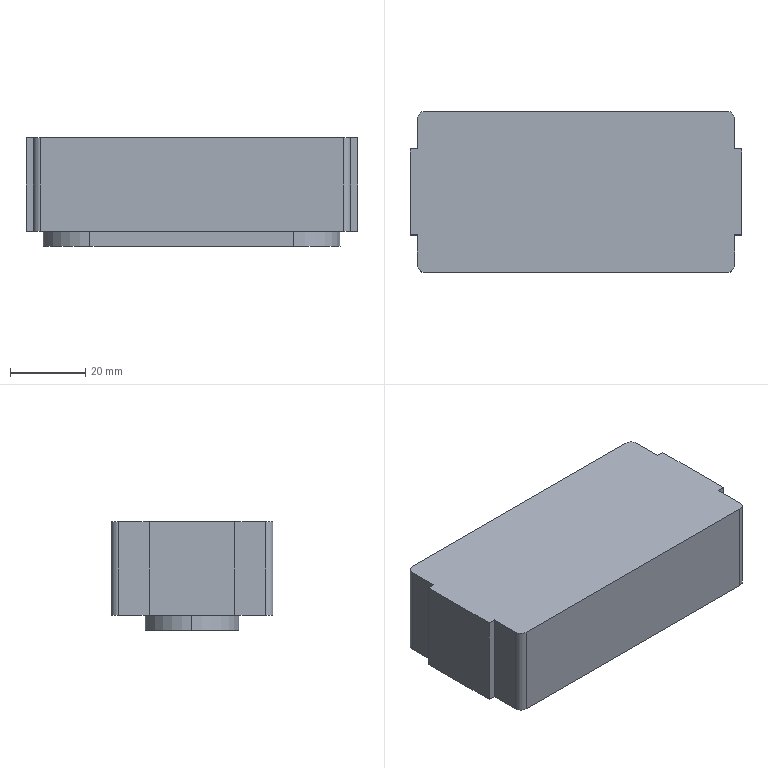Part | SolidWorks | features Extrusion 1, Fillet 1, ICE 1 | 1 solid | 24 faces | box 88.335 x 43.022 x 29 mm | volume 100368 mm3 | plane 17 | cylinder 7 | commonest cylinder face diameters 4 x4 24.966 x3
STEP:
#1=CARTESIAN_POINT('',(-39.672,0.,4.));
#2=VERTEX_POINT('',#1);
#3=CARTESIAN_POINT('',(-27.189,-12.483,4.));
#4=VERTEX_POINT('',#3);
#5=CARTESIAN_POINT('',(-27.189,0.,4.));
#6=DIRECTION('',(0.,0.,1.));
#7=DIRECTION('',(1.,0.,0.));
#8=AXIS2_PLACEMENT_3D('',#5,#6,#7);
#9=CIRCLE('',#8,12.483);
#10=EDGE_CURVE('',#2,#4,#9,.T.);
#11=ORIENTED_EDGE('',*,*,#10,.F.);
#12=CARTESIAN_POINT('',(-39.672,0.,0.));
#13=VERTEX_POINT('',#12);
#14=CARTESIAN_POINT('',(-39.672,0.,4.));
#15=DIRECTION('',(0.,0.,-1.));
#16=VECTOR('',#15,1000.);
#17=LINE('',#14,#16);
#18=EDGE_CURVE('',#2,#13,#17,.T.);
#19=ORIENTED_EDGE('',*,*,#18,.T.);
#20=CARTESIAN_POINT('',(-27.189,-12.483,0.));
#21=VERTEX_POINT('',#20);
#22=CARTESIAN_POINT('',(-27.189,0.,0.));
#23=DIRECTION('',(0.,0.,1.));
#24=DIRECTION('',(1.,0.,0.));
#25=AXIS2_PLACEMENT_3D('',#22,#23,#24);
#26=CIRCLE('',#25,12.483);
#27=EDGE_CURVE('',#13,#21,#26,.T.);
#28=ORIENTED_EDGE('',*,*,#27,.T.);
#29=CARTESIAN_POINT('',(-27.189,-12.483,4.));
#30=DIRECTION('',(0.,0.,-1.));
#31=VECTOR('',#30,1000.);
#32=LINE('',#29,#31);
#33=EDGE_CURVE('',#4,#21,#32,.T.);
#34=ORIENTED_EDGE('',*,*,#33,.F.);
#35=EDGE_LOOP('',(#11,#19,#28,#34));
#36=FACE_OUTER_BOUND('',#35,.T.);
#37=CARTESIAN_POINT('',(-27.189,0.,4.));
#38=DIRECTION('',(0.,0.,-1.));
#39=DIRECTION('',(-1.,0.,0.));
#40=AXIS2_PLACEMENT_3D('',#37,#38,#39);
#41=CYLINDRICAL_SURFACE('',#40,12.483);
#42=ADVANCED_FACE('',(#36),#41,.T.);
#43=CARTESIAN_POINT('',(27.066,-12.483,0.));
#44=VERTEX_POINT('',#43);
#45=CARTESIAN_POINT('',(27.066,12.483,0.));
#46=VERTEX_POINT('',#45);
#47=CARTESIAN_POINT('',(27.066,0.,0.));
#48=DIRECTION('',(0.,0.,1.));
#49=DIRECTION('',(1.,0.,0.));
#50=AXIS2_PLACEMENT_3D('',#47,#48,#49);
#51=CIRCLE('',#50,12.483);
#52=EDGE_CURVE('',#44,#46,#51,.T.);
#53=ORIENTED_EDGE('',*,*,#52,.T.);
#54=CARTESIAN_POINT('',(27.066,12.483,4.));
#55=VERTEX_POINT('',#54);
#56=CARTESIAN_POINT('',(27.066,12.483,4.));
#57=DIRECTION('',(0.,0.,-1.));
#58=VECTOR('',#57,1000.);
#59=LINE('',#56,#58);
#60=EDGE_CURVE('',#55,#46,#59,.T.);
#61=ORIENTED_EDGE('',*,*,#60,.F.);
#62=CARTESIAN_POINT('',(27.066,-12.483,4.));
#63=VERTEX_POINT('',#62);
#64=CARTESIAN_POINT('',(27.066,0.,4.));
#65=DIRECTION('',(0.,0.,1.));
#66=DIRECTION('',(1.,0.,0.));
#67=AXIS2_PLACEMENT_3D('',#64,#65,#66);
#68=CIRCLE('',#67,12.483);
#69=EDGE_CURVE('',#63,#55,#68,.T.);
#70=ORIENTED_EDGE('',*,*,#69,.F.);
#71=CARTESIAN_POINT('',(27.066,-12.483,4.));
#72=DIRECTION('',(0.,0.,-1.));
#73=VECTOR('',#72,1000.);
#74=LINE('',#71,#73);
#75=EDGE_CURVE('',#63,#44,#74,.T.);
#76=ORIENTED_EDGE('',*,*,#75,.T.);
#77=EDGE_LOOP('',(#53,#61,#70,#76));
#78=FACE_OUTER_BOUND('',#77,.T.);
#79=CARTESIAN_POINT('',(27.066,0.,4.));
#80=DIRECTION('',(0.,0.,-1.));
#81=DIRECTION('',(-1.,0.,0.));
#82=AXIS2_PLACEMENT_3D('',#79,#80,#81);
#83=CYLINDRICAL_SURFACE('',#82,12.483);
#84=ADVANCED_FACE('',(#78),#83,.T.);
#85=CARTESIAN_POINT('',(-27.189,12.483,0.));
#86=VERTEX_POINT('',#85);
#87=CARTESIAN_POINT('',(27.066,12.483,0.));
#88=DIRECTION('',(-1.,0.,0.));
#89=VECTOR('',#88,1000.);
#90=LINE('',#87,#89);
#91=EDGE_CURVE('',#46,#86,#90,.T.);
#92=ORIENTED_EDGE('',*,*,#91,.T.);
#93=CARTESIAN_POINT('',(-27.189,12.483,4.));
#94=VERTEX_POINT('',#93);
#95=CARTESIAN_POINT('',(-27.189,12.483,4.));
#96=DIRECTION('',(0.,0.,-1.));
#97=VECTOR('',#96,1000.);
#98=LINE('',#95,#97);
#99=EDGE_CURVE('',#94,#86,#98,.T.);
#100=ORIENTED_EDGE('',*,*,#99,.F.);
#101=CARTESIAN_POINT('',(27.066,12.483,4.));
#102=DIRECTION('',(-1.,0.,0.));
#103=VECTOR('',#102,1000.);
#104=LINE('',#101,#103);
#105=EDGE_CURVE('',#55,#94,#104,.T.);
#106=ORIENTED_EDGE('',*,*,#105,.F.);
#107=ORIENTED_EDGE('',*,*,#60,.T.);
#108=EDGE_LOOP('',(#92,#100,#106,#107));
#109=FACE_OUTER_BOUND('',#108,.T.);
#110=CARTESIAN_POINT('',(27.066,12.483,4.));
#111=DIRECTION('',(0.,-1.,0.));
#112=DIRECTION('',(1.,0.,0.));
#113=AXIS2_PLACEMENT_3D('',#110,#111,#112);
#114=PLANE('',#113);
#115=ADVANCED_FACE('',(#109),#114,.F.);
#116=ORIENTED_EDGE('',*,*,#18,.F.);
#117=CARTESIAN_POINT('',(-27.189,0.,4.));
#118=DIRECTION('',(0.,0.,1.));
#119=DIRECTION('',(1.,0.,0.));
#120=AXIS2_PLACEMENT_3D('',#117,#118,#119);
#121=CIRCLE('',#120,12.483);
#122=EDGE_CURVE('',#94,#2,#121,.T.);
#123=ORIENTED_EDGE('',*,*,#122,.F.);
#124=ORIENTED_EDGE('',*,*,#99,.T.);
#125=CARTESIAN_POINT('',(-27.189,0.,0.));
#126=DIRECTION('',(0.,0.,1.));
#127=DIRECTION('',(1.,0.,0.));
#128=AXIS2_PLACEMENT_3D('',#125,#126,#127);
#129=CIRCLE('',#128,12.483);
#130=EDGE_CURVE('',#86,#13,#129,.T.);
#131=ORIENTED_EDGE('',*,*,#130,.T.);
#132=EDGE_LOOP('',(#116,#123,#124,#131));
#133=FACE_OUTER_BOUND('',#132,.T.);
#134=CARTESIAN_POINT('',(-27.189,0.,4.));
#135=DIRECTION('',(0.,0.,-1.));
#136=DIRECTION('',(-1.,0.,0.));
#137=AXIS2_PLACEMENT_3D('',#134,#135,#136);
#138=CYLINDRICAL_SURFACE('',#137,12.483);
#139=ADVANCED_FACE('',(#133),#138,.T.);
#140=CARTESIAN_POINT('',(27.066,-12.483,0.));
#141=DIRECTION('',(1.,0.,0.));
#142=VECTOR('',#141,1000.);
#143=LINE('',#140,#142);
#144=EDGE_CURVE('',#21,#44,#143,.T.);
#145=ORIENTED_EDGE('',*,*,#144,.T.);
#146=ORIENTED_EDGE('',*,*,#75,.F.);
#147=CARTESIAN_POINT('',(27.066,-12.483,4.));
#148=DIRECTION('',(1.,0.,0.));
#149=VECTOR('',#148,1000.);
#150=LINE('',#147,#149);
#151=EDGE_CURVE('',#4,#63,#150,.T.);
#152=ORIENTED_EDGE('',*,*,#151,.F.);
#153=ORIENTED_EDGE('',*,*,#33,.T.);
#154=EDGE_LOOP('',(#145,#146,#152,#153));
#155=FACE_OUTER_BOUND('',#154,.T.);
#156=CARTESIAN_POINT('',(27.066,-12.483,4.));
#157=DIRECTION('',(0.,1.,0.));
#158=DIRECTION('',(-1.,0.,0.));
#159=AXIS2_PLACEMENT_3D('',#156,#157,#158);
#160=PLANE('',#159);
#161=ADVANCED_FACE('',(#155),#160,.F.);
#162=ORIENTED_EDGE('',*,*,#52,.F.);
#163=ORIENTED_EDGE('',*,*,#144,.F.);
#164=ORIENTED_EDGE('',*,*,#27,.F.);
#165=ORIENTED_EDGE('',*,*,#130,.F.);
#166=ORIENTED_EDGE('',*,*,#91,.F.);
#167=EDGE_LOOP('',(#162,#163,#164,#165,#166));
#168=FACE_OUTER_BOUND('',#167,.T.);
#169=CARTESIAN_POINT('',(27.066,0.,0.));
#170=DIRECTION('',(0.,0.,1.));
#171=DIRECTION('',(1.,0.,0.));
#172=AXIS2_PLACEMENT_3D('',#169,#170,#171);
#173=PLANE('',#172);
#174=ADVANCED_FACE('',(#168),#173,.F.);
#175=CARTESIAN_POINT('',(-42.249,19.511,4.));
#176=VERTEX_POINT('',#175);
#177=CARTESIAN_POINT('',(-42.249,11.445,4.));
#178=VERTEX_POINT('',#177);
#179=CARTESIAN_POINT('',(-42.249,11.445,4.));
#180=DIRECTION('',(0.,-1.,0.));
#181=VECTOR('',#180,1000.);
#182=LINE('',#179,#181);
#183=EDGE_CURVE('',#176,#178,#182,.T.);
#184=ORIENTED_EDGE('',*,*,#183,.F.);
#185=CARTESIAN_POINT('',(-40.249,21.511,4.));
#186=VERTEX_POINT('',#185);
#187=CARTESIAN_POINT('',(-40.249,19.511,4.));
#188=DIRECTION('',(0.,0.,-1.));
#189=DIRECTION('',(1.,0.,0.));
#190=AXIS2_PLACEMENT_3D('',#187,#188,#189);
#191=CIRCLE('',#190,2.);
#192=EDGE_CURVE('',#176,#186,#191,.T.);
#193=ORIENTED_EDGE('',*,*,#192,.T.);
#194=CARTESIAN_POINT('',(40.249,21.511,4.));
#195=VERTEX_POINT('',#194);
#196=CARTESIAN_POINT('',(42.249,21.511,4.));
#197=DIRECTION('',(-1.,0.,0.));
#198=VECTOR('',#197,1000.);
#199=LINE('',#196,#198);
#200=EDGE_CURVE('',#195,#186,#199,.T.);
#201=ORIENTED_EDGE('',*,*,#200,.F.);
#202=CARTESIAN_POINT('',(42.249,19.511,4.));
#203=VERTEX_POINT('',#202);
#204=CARTESIAN_POINT('',(40.249,19.511,4.));
#205=DIRECTION('',(0.,0.,-1.));
#206=DIRECTION('',(1.,0.,0.));
#207=AXIS2_PLACEMENT_3D('',#204,#205,#206);
#208=CIRCLE('',#207,2.);
#209=EDGE_CURVE('',#195,#203,#208,.T.);
#210=ORIENTED_EDGE('',*,*,#209,.T.);
#211=CARTESIAN_POINT('',(42.249,11.445,4.));
#212=VERTEX_POINT('',#211);
#213=CARTESIAN_POINT('',(42.249,11.445,4.));
#214=DIRECTION('',(0.,1.,0.));
#215=VECTOR('',#214,1000.);
#216=LINE('',#213,#215);
#217=EDGE_CURVE('',#212,#203,#216,.T.);
#218=ORIENTED_EDGE('',*,*,#217,.F.);
#219=CARTESIAN_POINT('',(44.167,11.445,4.));
#220=VERTEX_POINT('',#219);
#221=CARTESIAN_POINT('',(44.167,11.445,4.));
#222=DIRECTION('',(-1.,0.,0.));
#223=VECTOR('',#222,1000.);
#224=LINE('',#221,#223);
#225=EDGE_CURVE('',#220,#212,#224,.T.);
#226=ORIENTED_EDGE('',*,*,#225,.F.);
#227=CARTESIAN_POINT('',(44.167,-11.445,4.));
#228=VERTEX_POINT('',#227);
#229=CARTESIAN_POINT('',(44.167,-11.445,4.));
#230=DIRECTION('',(0.,1.,0.));
#231=VECTOR('',#230,1000.);
#232=LINE('',#229,#231);
#233=EDGE_CURVE('',#228,#220,#232,.T.);
#234=ORIENTED_EDGE('',*,*,#233,.F.);
#235=CARTESIAN_POINT('',(42.249,-11.445,4.));
#236=VERTEX_POINT('',#235);
#237=CARTESIAN_POINT('',(44.167,-11.445,4.));
#238=DIRECTION('',(1.,0.,0.));
#239=VECTOR('',#238,1000.);
#240=LINE('',#237,#239);
#241=EDGE_CURVE('',#236,#228,#240,.T.);
#242=ORIENTED_EDGE('',*,*,#241,.F.);
#243=CARTESIAN_POINT('',(42.249,-19.511,4.));
#244=VERTEX_POINT('',#243);
#245=CARTESIAN_POINT('',(42.249,-21.511,4.));
#246=DIRECTION('',(0.,1.,0.));
#247=VECTOR('',#246,1000.);
#248=LINE('',#245,#247);
#249=EDGE_CURVE('',#244,#236,#248,.T.);
#250=ORIENTED_EDGE('',*,*,#249,.F.);
#251=CARTESIAN_POINT('',(40.249,-21.511,4.));
#252=VERTEX_POINT('',#251);
#253=CARTESIAN_POINT('',(40.249,-19.511,4.));
#254=DIRECTION('',(0.,0.,-1.));
#255=DIRECTION('',(1.,0.,0.));
#256=AXIS2_PLACEMENT_3D('',#253,#254,#255);
#257=CIRCLE('',#256,2.);
#258=EDGE_CURVE('',#244,#252,#257,.T.);
#259=ORIENTED_EDGE('',*,*,#258,.T.);
#260=CARTESIAN_POINT('',(-40.249,-21.511,4.));
#261=VERTEX_POINT('',#260);
#262=CARTESIAN_POINT('',(42.249,-21.511,4.));
#263=DIRECTION('',(1.,0.,0.));
#264=VECTOR('',#263,1000.);
#265=LINE('',#262,#264);
#266=EDGE_CURVE('',#261,#252,#265,.T.);
#267=ORIENTED_EDGE('',*,*,#266,.F.);
#268=CARTESIAN_POINT('',(-42.249,-19.511,4.));
#269=VERTEX_POINT('',#268);
#270=CARTESIAN_POINT('',(-40.249,-19.511,4.));
#271=DIRECTION('',(0.,0.,-1.));
#272=DIRECTION('',(1.,0.,0.));
#273=AXIS2_PLACEMENT_3D('',#270,#271,#272);
#274=CIRCLE('',#273,2.);
#275=EDGE_CURVE('',#261,#269,#274,.T.);
#276=ORIENTED_EDGE('',*,*,#275,.T.);
#277=CARTESIAN_POINT('',(-42.249,-11.445,4.));
#278=VERTEX_POINT('',#277);
#279=CARTESIAN_POINT('',(-42.249,-21.511,4.));
#280=DIRECTION('',(0.,-1.,0.));
#281=VECTOR('',#280,1000.);
#282=LINE('',#279,#281);
#283=EDGE_CURVE('',#278,#269,#282,.T.);
#284=ORIENTED_EDGE('',*,*,#283,.F.);
#285=CARTESIAN_POINT('',(-44.167,-11.445,4.));
#286=VERTEX_POINT('',#285);
#287=CARTESIAN_POINT('',(-44.167,-11.445,4.));
#288=DIRECTION('',(1.,0.,0.));
#289=VECTOR('',#288,1000.);
#290=LINE('',#287,#289);
#291=EDGE_CURVE('',#286,#278,#290,.T.);
#292=ORIENTED_EDGE('',*,*,#291,.F.);
#293=CARTESIAN_POINT('',(-44.167,11.445,4.));
#294=VERTEX_POINT('',#293);
#295=CARTESIAN_POINT('',(-44.167,-11.445,4.));
#296=DIRECTION('',(0.,-1.,0.));
#297=VECTOR('',#296,1000.);
#298=LINE('',#295,#297);
#299=EDGE_CURVE('',#294,#286,#298,.T.);
#300=ORIENTED_EDGE('',*,*,#299,.F.);
#301=CARTESIAN_POINT('',(-44.167,11.445,4.));
#302=DIRECTION('',(-1.,0.,0.));
#303=VECTOR('',#302,1000.);
#304=LINE('',#301,#303);
#305=EDGE_CURVE('',#178,#294,#304,.T.);
#306=ORIENTED_EDGE('',*,*,#305,.F.);
#307=EDGE_LOOP('',(#184,#193,#201,#210,#218,#226,#234,#242,#250,#259,#267,#276,#284,#292,#300,#306));
#308=FACE_OUTER_BOUND('',#307,.T.);
#309=ORIENTED_EDGE('',*,*,#151,.T.);
#310=ORIENTED_EDGE('',*,*,#69,.T.);
#311=ORIENTED_EDGE('',*,*,#105,.T.);
#312=ORIENTED_EDGE('',*,*,#122,.T.);
#313=ORIENTED_EDGE('',*,*,#10,.T.);
#314=EDGE_LOOP('',(#309,#310,#311,#312,#313));
#315=FACE_BOUND('',#314,.T.);
#316=CARTESIAN_POINT('',(0.,0.,4.));
#317=DIRECTION('',(0.,0.,1.));
#318=DIRECTION('',(1.,0.,0.));
#319=AXIS2_PLACEMENT_3D('',#316,#317,#318);
#320=PLANE('',#319);
#321=ADVANCED_FACE('',(#308,#315),#320,.F.);
#322=CARTESIAN_POINT('',(-42.249,19.511,29.));
#323=VERTEX_POINT('',#322);
#324=CARTESIAN_POINT('',(-42.249,11.445,29.));
#325=VERTEX_POINT('',#324);
#326=CARTESIAN_POINT('',(-42.249,11.445,29.));
#327=DIRECTION('',(0.,-1.,0.));
#328=VECTOR('',#327,1000.);
#329=LINE('',#326,#328);
#330=EDGE_CURVE('',#323,#325,#329,.T.);
#331=ORIENTED_EDGE('',*,*,#330,.F.);
#332=CARTESIAN_POINT('',(-42.249,19.511,29.));
#333=DIRECTION('',(0.,0.,-1.));
#334=VECTOR('',#333,1000.);
#335=LINE('',#332,#334);
#336=EDGE_CURVE('',#323,#176,#335,.T.);
#337=ORIENTED_EDGE('',*,*,#336,.T.);
#338=ORIENTED_EDGE('',*,*,#183,.T.);
#339=CARTESIAN_POINT('',(-42.249,11.445,29.));
#340=DIRECTION('',(0.,0.,-1.));
#341=VECTOR('',#340,1000.);
#342=LINE('',#339,#341);
#343=EDGE_CURVE('',#325,#178,#342,.T.);
#344=ORIENTED_EDGE('',*,*,#343,.F.);
#345=EDGE_LOOP('',(#331,#337,#338,#344));
#346=FACE_OUTER_BOUND('',#345,.T.);
#347=CARTESIAN_POINT('',(-42.249,11.445,29.));
#348=DIRECTION('',(1.,0.,0.));
#349=DIRECTION('',(0.,0.,-1.));
#350=AXIS2_PLACEMENT_3D('',#347,#348,#349);
#351=PLANE('',#350);
#352=ADVANCED_FACE('',(#346),#351,.F.);
#353=ORIENTED_EDGE('',*,*,#305,.T.);
#354=CARTESIAN_POINT('',(-44.167,11.445,29.));
#355=VERTEX_POINT('',#354);
#356=CARTESIAN_POINT('',(-44.167,11.445,29.));
#357=DIRECTION('',(0.,0.,-1.));
#358=VECTOR('',#357,1000.);
#359=LINE('',#356,#358);
#360=EDGE_CURVE('',#355,#294,#359,.T.);
#361=ORIENTED_EDGE('',*,*,#360,.F.);
#362=CARTESIAN_POINT('',(-44.167,11.445,29.));
#363=DIRECTION('',(-1.,0.,0.));
#364=VECTOR('',#363,1000.);
#365=LINE('',#362,#364);
#366=EDGE_CURVE('',#325,#355,#365,.T.);
#367=ORIENTED_EDGE('',*,*,#366,.F.);
#368=ORIENTED_EDGE('',*,*,#343,.T.);
#369=EDGE_LOOP('',(#353,#361,#367,#368));
#370=FACE_OUTER_BOUND('',#369,.T.);
#371=CARTESIAN_POINT('',(-44.167,11.445,29.));
#372=DIRECTION('',(0.,-1.,0.));
#373=DIRECTION('',(1.,0.,0.));
#374=AXIS2_PLACEMENT_3D('',#371,#372,#373);
#375=PLANE('',#374);
#376=ADVANCED_FACE('',(#370),#375,.F.);
#377=ORIENTED_EDGE('',*,*,#299,.T.);
#378=CARTESIAN_POINT('',(-44.167,-11.445,29.));
#379=VERTEX_POINT('',#378);
#380=CARTESIAN_POINT('',(-44.167,-11.445,29.));
#381=DIRECTION('',(0.,0.,-1.));
#382=VECTOR('',#381,1000.);
#383=LINE('',#380,#382);
#384=EDGE_CURVE('',#379,#286,#383,.T.);
#385=ORIENTED_EDGE('',*,*,#384,.F.);
#386=CARTESIAN_POINT('',(-44.167,-11.445,29.));
#387=DIRECTION('',(0.,-1.,0.));
#388=VECTOR('',#387,1000.);
#389=LINE('',#386,#388);
#390=EDGE_CURVE('',#355,#379,#389,.T.);
#391=ORIENTED_EDGE('',*,*,#390,.F.);
#392=ORIENTED_EDGE('',*,*,#360,.T.);
#393=EDGE_LOOP('',(#377,#385,#391,#392));
#394=FACE_OUTER_BOUND('',#393,.T.);
#395=CARTESIAN_POINT('',(-44.167,-11.445,29.));
#396=DIRECTION('',(1.,0.,0.));
#397=DIRECTION('',(0.,0.,-1.));
#398=AXIS2_PLACEMENT_3D('',#395,#396,#397);
#399=PLANE('',#398);
#400=ADVANCED_FACE('',(#394),#399,.F.);
#401=ORIENTED_EDGE('',*,*,#291,.T.);
#402=CARTESIAN_POINT('',(-42.249,-11.445,29.));
#403=VERTEX_POINT('',#402);
#404=CARTESIAN_POINT('',(-42.249,-11.445,29.));
#405=DIRECTION('',(0.,0.,-1.));
#406=VECTOR('',#405,1000.);
#407=LINE('',#404,#406);
#408=EDGE_CURVE('',#403,#278,#407,.T.);
#409=ORIENTED_EDGE('',*,*,#408,.F.);
#410=CARTESIAN_POINT('',(-44.167,-11.445,29.));
#411=DIRECTION('',(1.,0.,0.));
#412=VECTOR('',#411,1000.);
#413=LINE('',#410,#412);
#414=EDGE_CURVE('',#379,#403,#413,.T.);
#415=ORIENTED_EDGE('',*,*,#414,.F.);
#416=ORIENTED_EDGE('',*,*,#384,.T.);
#417=EDGE_LOOP('',(#401,#409,#415,#416));
#418=FACE_OUTER_BOUND('',#417,.T.);
#419=CARTESIAN_POINT('',(-44.167,-11.445,29.));
#420=DIRECTION('',(0.,1.,0.));
#421=DIRECTION('',(0.,0.,1.));
#422=AXIS2_PLACEMENT_3D('',#419,#420,#421);
#423=PLANE('',#422);
#424=ADVANCED_FACE('',(#418),#423,.F.);
#425=ORIENTED_EDGE('',*,*,#283,.T.);
#426=CARTESIAN_POINT('',(-42.249,-19.511,29.));
#427=VERTEX_POINT('',#426);
#428=CARTESIAN_POINT('',(-42.249,-19.511,29.));
#429=DIRECTION('',(0.,0.,1.));
#430=VECTOR('',#429,1000.);
#431=LINE('',#428,#430);
#432=EDGE_CURVE('',#269,#427,#431,.T.);
#433=ORIENTED_EDGE('',*,*,#432,.T.);
#434=CARTESIAN_POINT('',(-42.249,-21.511,29.));
#435=DIRECTION('',(0.,-1.,0.));
#436=VECTOR('',#435,1000.);
#437=LINE('',#434,#436);
#438=EDGE_CURVE('',#403,#427,#437,.T.);
#439=ORIENTED_EDGE('',*,*,#438,.F.);
#440=ORIENTED_EDGE('',*,*,#408,.T.);
#441=EDGE_LOOP('',(#425,#433,#439,#440));
#442=FACE_OUTER_BOUND('',#441,.T.);
#443=CARTESIAN_POINT('',(-42.249,-21.511,29.));
#444=DIRECTION('',(1.,0.,0.));
#445=DIRECTION('',(0.,0.,-1.));
#446=AXIS2_PLACEMENT_3D('',#443,#444,#445);
#447=PLANE('',#446);
#448=ADVANCED_FACE('',(#442),#447,.F.);
#449=CARTESIAN_POINT('',(-40.249,-21.511,29.));
#450=VERTEX_POINT('',#449);
#451=CARTESIAN_POINT('',(40.249,-21.511,29.));
#452=VERTEX_POINT('',#451);
#453=CARTESIAN_POINT('',(42.249,-21.511,29.));
#454=DIRECTION('',(1.,0.,0.));
#455=VECTOR('',#454,1000.);
#456=LINE('',#453,#455);
#457=EDGE_CURVE('',#450,#452,#456,.T.);
#458=ORIENTED_EDGE('',*,*,#457,.F.);
#459=CARTESIAN_POINT('',(-40.249,-21.511,29.));
#460=DIRECTION('',(0.,0.,-1.));
#461=VECTOR('',#460,1000.);
#462=LINE('',#459,#461);
#463=EDGE_CURVE('',#450,#261,#462,.T.);
#464=ORIENTED_EDGE('',*,*,#463,.T.);
#465=ORIENTED_EDGE('',*,*,#266,.T.);
#466=CARTESIAN_POINT('',(40.249,-21.511,29.));
#467=DIRECTION('',(0.,0.,1.));
#468=VECTOR('',#467,1000.);
#469=LINE('',#466,#468);
#470=EDGE_CURVE('',#252,#452,#469,.T.);
#471=ORIENTED_EDGE('',*,*,#470,.T.);
#472=EDGE_LOOP('',(#458,#464,#465,#471));
#473=FACE_OUTER_BOUND('',#472,.T.);
#474=CARTESIAN_POINT('',(42.249,-21.511,29.));
#475=DIRECTION('',(0.,1.,0.));
#476=DIRECTION('',(0.,0.,1.));
#477=AXIS2_PLACEMENT_3D('',#474,#475,#476);
#478=PLANE('',#477);
#479=ADVANCED_FACE('',(#473),#478,.F.);
#480=CARTESIAN_POINT('',(42.249,-19.511,29.));
#481=VERTEX_POINT('',#480);
#482=CARTESIAN_POINT('',(42.249,-11.445,29.));
#483=VERTEX_POINT('',#482);
#484=CARTESIAN_POINT('',(42.249,-21.511,29.));
#485=DIRECTION('',(0.,1.,0.));
#486=VECTOR('',#485,1000.);
#487=LINE('',#484,#486);
#488=EDGE_CURVE('',#481,#483,#487,.T.);
#489=ORIENTED_EDGE('',*,*,#488,.F.);
#490=CARTESIAN_POINT('',(42.249,-19.511,29.));
#491=DIRECTION('',(0.,0.,-1.));
#492=VECTOR('',#491,1000.);
#493=LINE('',#490,#492);
#494=EDGE_CURVE('',#481,#244,#493,.T.);
#495=ORIENTED_EDGE('',*,*,#494,.T.);
#496=ORIENTED_EDGE('',*,*,#249,.T.);
#497=CARTESIAN_POINT('',(42.249,-11.445,29.));
#498=DIRECTION('',(0.,0.,-1.));
#499=VECTOR('',#498,1000.);
#500=LINE('',#497,#499);
#501=EDGE_CURVE('',#483,#236,#500,.T.);
#502=ORIENTED_EDGE('',*,*,#501,.F.);
#503=EDGE_LOOP('',(#489,#495,#496,#502));
#504=FACE_OUTER_BOUND('',#503,.T.);
#505=CARTESIAN_POINT('',(42.249,-21.511,29.));
#506=DIRECTION('',(-1.,0.,0.));
#507=DIRECTION('',(0.,0.,1.));
#508=AXIS2_PLACEMENT_3D('',#505,#506,#507);
#509=PLANE('',#508);
#510=ADVANCED_FACE('',(#504),#509,.F.);
#511=ORIENTED_EDGE('',*,*,#241,.T.);
#512=CARTESIAN_POINT('',(44.167,-11.445,29.));
#513=VERTEX_POINT('',#512);
#514=CARTESIAN_POINT('',(44.167,-11.445,29.));
#515=DIRECTION('',(0.,0.,-1.));
#516=VECTOR('',#515,1000.);
#517=LINE('',#514,#516);
#518=EDGE_CURVE('',#513,#228,#517,.T.);
#519=ORIENTED_EDGE('',*,*,#518,.F.);
#520=CARTESIAN_POINT('',(44.167,-11.445,29.));
#521=DIRECTION('',(1.,0.,0.));
#522=VECTOR('',#521,1000.);
#523=LINE('',#520,#522);
#524=EDGE_CURVE('',#483,#513,#523,.T.);
#525=ORIENTED_EDGE('',*,*,#524,.F.);
#526=ORIENTED_EDGE('',*,*,#501,.T.);
#527=EDGE_LOOP('',(#511,#519,#525,#526));
#528=FACE_OUTER_BOUND('',#527,.T.);
#529=CARTESIAN_POINT('',(44.167,-11.445,29.));
#530=DIRECTION('',(0.,1.,0.));
#531=DIRECTION('',(0.,0.,1.));
#532=AXIS2_PLACEMENT_3D('',#529,#530,#531);
#533=PLANE('',#532);
#534=ADVANCED_FACE('',(#528),#533,.F.);
#535=ORIENTED_EDGE('',*,*,#233,.T.);
#536=CARTESIAN_POINT('',(44.167,11.445,29.));
#537=VERTEX_POINT('',#536);
#538=CARTESIAN_POINT('',(44.167,11.445,29.));
#539=DIRECTION('',(0.,0.,-1.));
#540=VECTOR('',#539,1000.);
#541=LINE('',#538,#540);
#542=EDGE_CURVE('',#537,#220,#541,.T.);
#543=ORIENTED_EDGE('',*,*,#542,.F.);
#544=CARTESIAN_POINT('',(44.167,-11.445,29.));
#545=DIRECTION('',(0.,1.,0.));
#546=VECTOR('',#545,1000.);
#547=LINE('',#544,#546);
#548=EDGE_CURVE('',#513,#537,#547,.T.);
#549=ORIENTED_EDGE('',*,*,#548,.F.);
#550=ORIENTED_EDGE('',*,*,#518,.T.);
#551=EDGE_LOOP('',(#535,#543,#549,#550));
#552=FACE_OUTER_BOUND('',#551,.T.);
#553=CARTESIAN_POINT('',(44.167,-11.445,29.));
#554=DIRECTION('',(-1.,0.,0.));
#555=DIRECTION('',(0.,0.,1.));
#556=AXIS2_PLACEMENT_3D('',#553,#554,#555);
#557=PLANE('',#556);
#558=ADVANCED_FACE('',(#552),#557,.F.);
#559=ORIENTED_EDGE('',*,*,#225,.T.);
#560=CARTESIAN_POINT('',(42.249,11.445,29.));
#561=VERTEX_POINT('',#560);
#562=CARTESIAN_POINT('',(42.249,11.445,29.));
#563=DIRECTION('',(0.,0.,-1.));
#564=VECTOR('',#563,1000.);
#565=LINE('',#562,#564);
#566=EDGE_CURVE('',#561,#212,#565,.T.);
#567=ORIENTED_EDGE('',*,*,#566,.F.);
#568=CARTESIAN_POINT('',(44.167,11.445,29.));
#569=DIRECTION('',(-1.,0.,0.));
#570=VECTOR('',#569,1000.);
#571=LINE('',#568,#570);
#572=EDGE_CURVE('',#537,#561,#571,.T.);
#573=ORIENTED_EDGE('',*,*,#572,.F.);
#574=ORIENTED_EDGE('',*,*,#542,.T.);
#575=EDGE_LOOP('',(#559,#567,#573,#574));
#576=FACE_OUTER_BOUND('',#575,.T.);
#577=CARTESIAN_POINT('',(44.167,11.445,29.));
#578=DIRECTION('',(0.,-1.,0.));
#579=DIRECTION('',(1.,0.,0.));
#580=AXIS2_PLACEMENT_3D('',#577,#578,#579);
#581=PLANE('',#580);
#582=ADVANCED_FACE('',(#576),#581,.F.);
#583=ORIENTED_EDGE('',*,*,#217,.T.);
#584=CARTESIAN_POINT('',(42.249,19.511,29.));
#585=VERTEX_POINT('',#584);
#586=CARTESIAN_POINT('',(42.249,19.511,29.));
#587=DIRECTION('',(0.,0.,1.));
#588=VECTOR('',#587,1000.);
#589=LINE('',#586,#588);
#590=EDGE_CURVE('',#203,#585,#589,.T.);
#591=ORIENTED_EDGE('',*,*,#590,.T.);
#592=CARTESIAN_POINT('',(42.249,11.445,29.));
#593=DIRECTION('',(0.,1.,0.));
#594=VECTOR('',#593,1000.);
#595=LINE('',#592,#594);
#596=EDGE_CURVE('',#561,#585,#595,.T.);
#597=ORIENTED_EDGE('',*,*,#596,.F.);
#598=ORIENTED_EDGE('',*,*,#566,.T.);
#599=EDGE_LOOP('',(#583,#591,#597,#598));
#600=FACE_OUTER_BOUND('',#599,.T.);
#601=CARTESIAN_POINT('',(42.249,11.445,29.));
#602=DIRECTION('',(-1.,0.,0.));
#603=DIRECTION('',(0.,0.,1.));
#604=AXIS2_PLACEMENT_3D('',#601,#602,#603);
#605=PLANE('',#604);
#606=ADVANCED_FACE('',(#600),#605,.F.);
#607=ORIENTED_EDGE('',*,*,#200,.T.);
#608=CARTESIAN_POINT('',(-40.249,21.511,29.));
#609=VERTEX_POINT('',#608);
#610=CARTESIAN_POINT('',(-40.249,21.511,29.));
#611=DIRECTION('',(0.,0.,1.));
#612=VECTOR('',#611,1000.);
#613=LINE('',#610,#612);
#614=EDGE_CURVE('',#186,#609,#613,.T.);
#615=ORIENTED_EDGE('',*,*,#614,.T.);
#616=CARTESIAN_POINT('',(40.249,21.511,29.));
#617=VERTEX_POINT('',#616);
#618=CARTESIAN_POINT('',(42.249,21.511,29.));
#619=DIRECTION('',(-1.,0.,0.));
#620=VECTOR('',#619,1000.);
#621=LINE('',#618,#620);
#622=EDGE_CURVE('',#617,#609,#621,.T.);
#623=ORIENTED_EDGE('',*,*,#622,.F.);
#624=CARTESIAN_POINT('',(40.249,21.511,29.));
#625=DIRECTION('',(0.,0.,-1.));
#626=VECTOR('',#625,1000.);
#627=LINE('',#624,#626);
#628=EDGE_CURVE('',#617,#195,#627,.T.);
#629=ORIENTED_EDGE('',*,*,#628,.T.);
#630=EDGE_LOOP('',(#607,#615,#623,#629));
#631=FACE_OUTER_BOUND('',#630,.T.);
#632=CARTESIAN_POINT('',(42.249,21.511,29.));
#633=DIRECTION('',(0.,-1.,0.));
#634=DIRECTION('',(0.,0.,-1.));
#635=AXIS2_PLACEMENT_3D('',#632,#633,#634);
#636=PLANE('',#635);
#637=ADVANCED_FACE('',(#631),#636,.F.);
#638=ORIENTED_EDGE('',*,*,#622,.T.);
#639=CARTESIAN_POINT('',(-40.249,19.511,29.));
#640=DIRECTION('',(0.,0.,1.));
#641=DIRECTION('',(1.,0.,0.));
#642=AXIS2_PLACEMENT_3D('',#639,#640,#641);
#643=CIRCLE('',#642,2.);
#644=EDGE_CURVE('',#609,#323,#643,.T.);
#645=ORIENTED_EDGE('',*,*,#644,.T.);
#646=ORIENTED_EDGE('',*,*,#330,.T.);
#647=ORIENTED_EDGE('',*,*,#366,.T.);
#648=ORIENTED_EDGE('',*,*,#390,.T.);
#649=ORIENTED_EDGE('',*,*,#414,.T.);
#650=ORIENTED_EDGE('',*,*,#438,.T.);
#651=CARTESIAN_POINT('',(-40.249,-19.511,29.));
#652=DIRECTION('',(0.,0.,1.));
#653=DIRECTION('',(1.,0.,0.));
#654=AXIS2_PLACEMENT_3D('',#651,#652,#653);
#655=CIRCLE('',#654,2.);
#656=EDGE_CURVE('',#427,#450,#655,.T.);
#657=ORIENTED_EDGE('',*,*,#656,.T.);
#658=ORIENTED_EDGE('',*,*,#457,.T.);
#659=CARTESIAN_POINT('',(40.249,-19.511,29.));
#660=DIRECTION('',(0.,0.,1.));
#661=DIRECTION('',(1.,0.,0.));
#662=AXIS2_PLACEMENT_3D('',#659,#660,#661);
#663=CIRCLE('',#662,2.);
#664=EDGE_CURVE('',#452,#481,#663,.T.);
#665=ORIENTED_EDGE('',*,*,#664,.T.);
#666=ORIENTED_EDGE('',*,*,#488,.T.);
#667=ORIENTED_EDGE('',*,*,#524,.T.);
#668=ORIENTED_EDGE('',*,*,#548,.T.);
#669=ORIENTED_EDGE('',*,*,#572,.T.);
#670=ORIENTED_EDGE('',*,*,#596,.T.);
#671=CARTESIAN_POINT('',(40.249,19.511,29.));
#672=DIRECTION('',(0.,0.,1.));
#673=DIRECTION('',(1.,0.,0.));
#674=AXIS2_PLACEMENT_3D('',#671,#672,#673);
#675=CIRCLE('',#674,2.);
#676=EDGE_CURVE('',#585,#617,#675,.T.);
#677=ORIENTED_EDGE('',*,*,#676,.T.);
#678=EDGE_LOOP('',(#638,#645,#646,#647,#648,#649,#650,#657,#658,#665,#666,#667,#668,#669,#670,#677));
#679=FACE_OUTER_BOUND('',#678,.T.);
#680=CARTESIAN_POINT('',(0.,0.,29.));
#681=DIRECTION('',(0.,0.,1.));
#682=DIRECTION('',(1.,0.,0.));
#683=AXIS2_PLACEMENT_3D('',#680,#681,#682);
#684=PLANE('',#683);
#685=ADVANCED_FACE('',(#679),#684,.T.);
#686=ORIENTED_EDGE('',*,*,#644,.F.);
#687=ORIENTED_EDGE('',*,*,#614,.F.);
#688=ORIENTED_EDGE('',*,*,#192,.F.);
#689=ORIENTED_EDGE('',*,*,#336,.F.);
#690=EDGE_LOOP('',(#686,#687,#688,#689));
#691=FACE_OUTER_BOUND('',#690,.T.);
#692=CARTESIAN_POINT('',(-40.249,19.511,29.));
#693=DIRECTION('',(0.,0.,-1.));
#694=DIRECTION('',(-1.,0.,0.));
#695=AXIS2_PLACEMENT_3D('',#692,#693,#694);
#696=CYLINDRICAL_SURFACE('',#695,2.);
#697=ADVANCED_FACE('',(#691),#696,.T.);
#698=ORIENTED_EDGE('',*,*,#656,.F.);
#699=ORIENTED_EDGE('',*,*,#432,.F.);
#700=ORIENTED_EDGE('',*,*,#275,.F.);
#701=ORIENTED_EDGE('',*,*,#463,.F.);
#702=EDGE_LOOP('',(#698,#699,#700,#701));
#703=FACE_OUTER_BOUND('',#702,.T.);
#704=CARTESIAN_POINT('',(-40.249,-19.511,29.));
#705=DIRECTION('',(0.,0.,-1.));
#706=DIRECTION('',(-1.,0.,0.));
#707=AXIS2_PLACEMENT_3D('',#704,#705,#706);
#708=CYLINDRICAL_SURFACE('',#707,2.);
#709=ADVANCED_FACE('',(#703),#708,.T.);
#710=ORIENTED_EDGE('',*,*,#676,.F.);
#711=ORIENTED_EDGE('',*,*,#590,.F.);
#712=ORIENTED_EDGE('',*,*,#209,.F.);
#713=ORIENTED_EDGE('',*,*,#628,.F.);
#714=EDGE_LOOP('',(#710,#711,#712,#713));
#715=FACE_OUTER_BOUND('',#714,.T.);
#716=CARTESIAN_POINT('',(40.249,19.511,29.));
#717=DIRECTION('',(0.,0.,-1.));
#718=DIRECTION('',(-1.,0.,0.));
#719=AXIS2_PLACEMENT_3D('',#716,#717,#718);
#720=CYLINDRICAL_SURFACE('',#719,2.);
#721=ADVANCED_FACE('',(#715),#720,.T.);
#722=ORIENTED_EDGE('',*,*,#664,.F.);
#723=ORIENTED_EDGE('',*,*,#470,.F.);
#724=ORIENTED_EDGE('',*,*,#258,.F.);
#725=ORIENTED_EDGE('',*,*,#494,.F.);
#726=EDGE_LOOP('',(#722,#723,#724,#725));
#727=FACE_OUTER_BOUND('',#726,.T.);
#728=CARTESIAN_POINT('',(40.249,-19.511,29.));
#729=DIRECTION('',(0.,0.,-1.));
#730=DIRECTION('',(-1.,0.,0.));
#731=AXIS2_PLACEMENT_3D('',#728,#729,#730);
#732=CYLINDRICAL_SURFACE('',#731,2.);
#733=ADVANCED_FACE('',(#727),#732,.T.);
#734=CLOSED_SHELL('',(#42,#84,#115,#139,#161,#174,#321,#352,#376,#400,#424,#448,#479,#510,#534,#558,#582,#606,#637,#685,#697,#709,#721,#733));
#735=MANIFOLD_SOLID_BREP('',#734);
#736=CARTESIAN_POINT('',(0.,0.,0.));
#737=DIRECTION('',(0.,0.,1.));
#738=DIRECTION('',(1.,0.,0.));
#739=AXIS2_PLACEMENT_3D('',#736,#737,#738);
#740=(LENGTH_UNIT()NAMED_UNIT(*)SI_UNIT(.MILLI.,.METRE.));
#741=UNCERTAINTY_MEASURE_WITH_UNIT(LENGTH_MEASURE(0.00001),#740,'','');
#742=(NAMED_UNIT(*)PLANE_ANGLE_UNIT()SI_UNIT($,.RADIAN.));
#743=(NAMED_UNIT(*)SI_UNIT($,.STERADIAN.)SOLID_ANGLE_UNIT());
#744=(GEOMETRIC_REPRESENTATION_CONTEXT(3)GLOBAL_UNCERTAINTY_ASSIGNED_CONTEXT((#741))GLOBAL_UNIT_ASSIGNED_CONTEXT((#740,#742,#743))REPRESENTATION_CONTEXT('',''));
#745=ADVANCED_BREP_SHAPE_REPRESENTATION('',(#735,#739),#744);